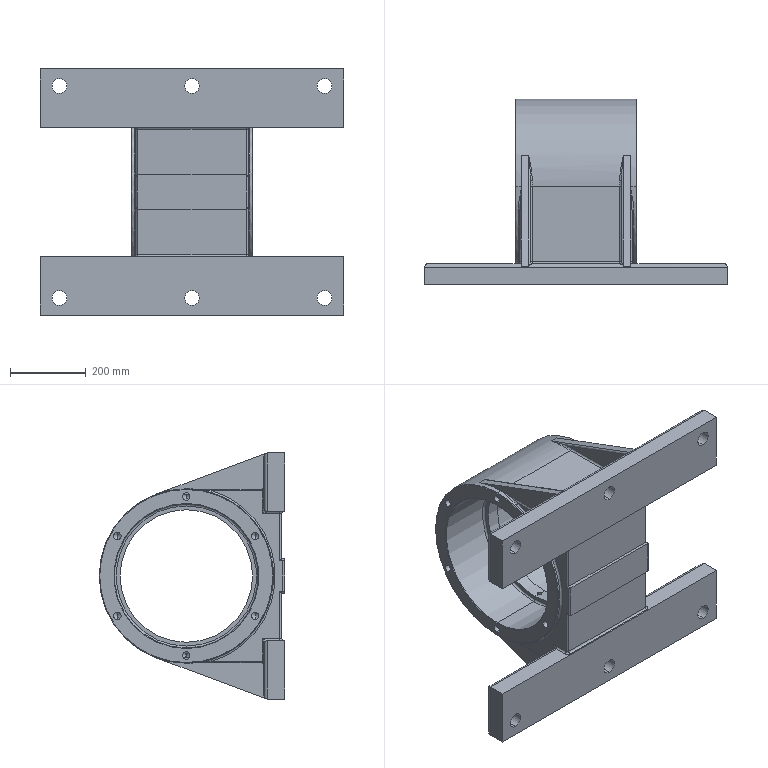Part | SolidWorks | features ICE 6, Fillet 4, MirrorPattern 3, 3DProfileFeature 2, HoleWzd 2, LPattern 2, Chamfer 1, CirPattern 1, Revolution 1 | 1 solid | 243 faces | box 800 x 490 x 650 mm | volume 39850758 mm3 | cylinder 109 | plane 60 | cone 32 | spline 20 | torus 18 | sphere 4 | commonest cylinder face diameters 10 x38 19.446 x24 39 x12 60 x12 20 x10 380 x4